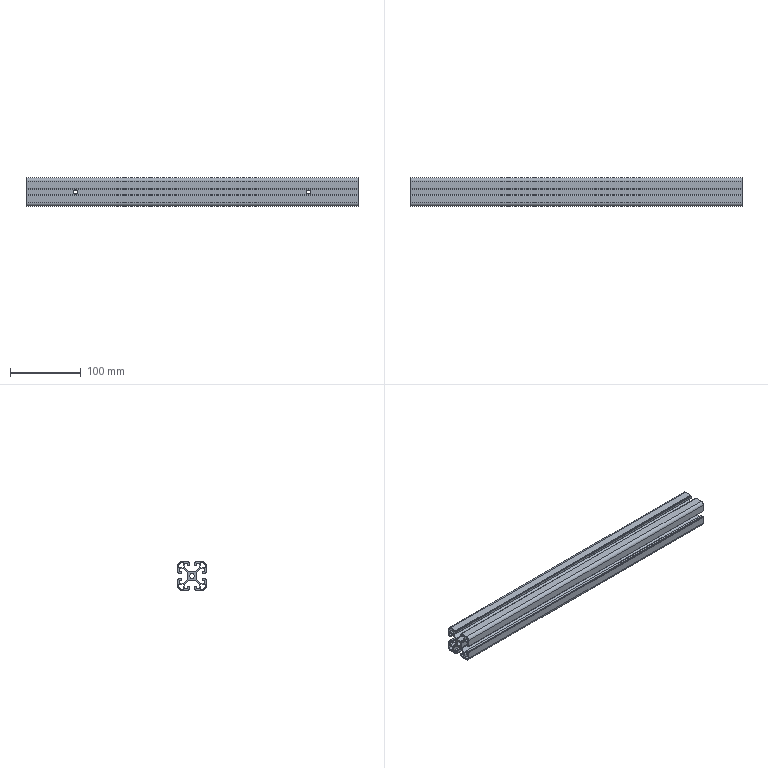Part | STEP file | 1 solid | 226 faces | box 470 x 40 x 40 mm | volume 224394 mm3 | cylinder 120 | plane 106 | commonest cylinder face diameters 0.6 x38 2 x28 4 x16 10 x10 0.4 x8 5.8 x8